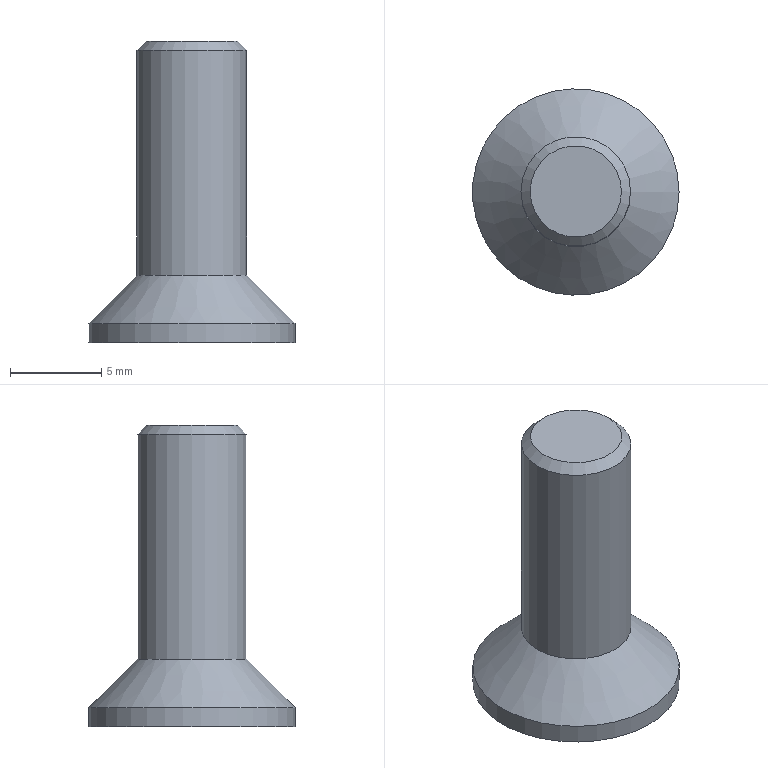Part | STEP file | solid 27 | 1 solid | 13 faces | box 11.3 x 11.3 x 16.5 mm | volume 595.104 mm3 | plane 9 | cylinder 2 | cone 2 | commonest cylinder face diameters 6 x1 11.3 x1